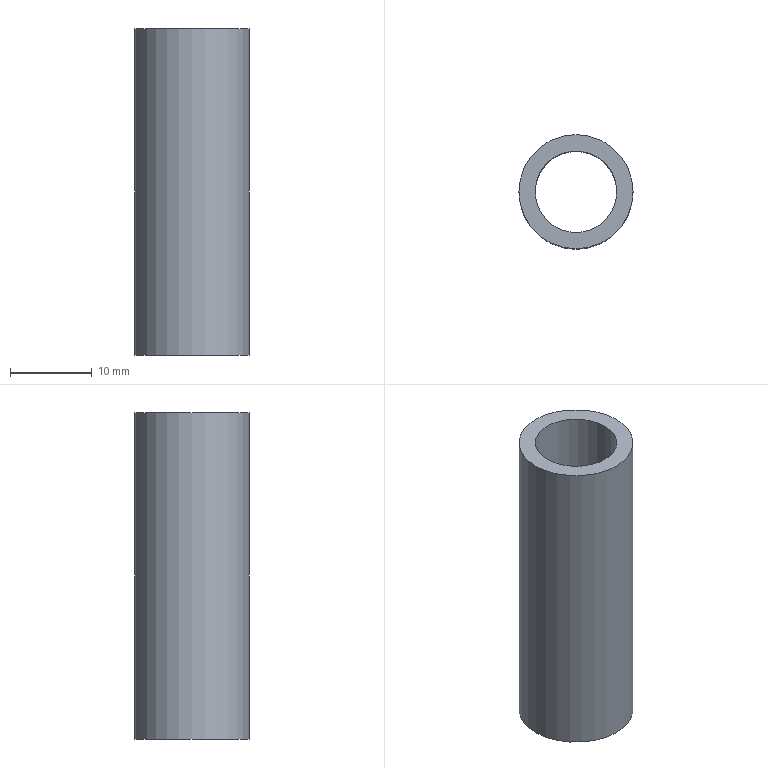Part | NX | features solid 2 | 1 solid | 4 faces | box 14 x 14 x 40 mm | volume 3016 mm3 | cylinder 2 | plane 2 | commonest cylinder face diameters 10 x1 14 x1
STEP:
#1=CARTESIAN_POINT('',(-1230.,410.,3.));
#2=VERTEX_POINT('',#1);
#3=CARTESIAN_POINT('',(-1225.,410.,3.));
#4=DIRECTION('',(0.,0.,-1.));
#5=DIRECTION('',(-1.,0.,0.));
#6=AXIS2_PLACEMENT_3D('',#3,#4,#5);
#7=CIRCLE('',#6,5.);
#8=EDGE_CURVE('',#2,#2,#7,.T.);
#9=ORIENTED_EDGE('',*,*,#8,.T.);
#10=EDGE_LOOP('',(#9));
#11=FACE_BOUND('',#10,.T.);
#12=CARTESIAN_POINT('',(-1230.,410.,43.));
#13=VERTEX_POINT('',#12);
#14=CARTESIAN_POINT('',(-1225.,410.,43.));
#15=DIRECTION('',(0.,0.,-1.));
#16=DIRECTION('',(-1.,0.,0.));
#17=AXIS2_PLACEMENT_3D('',#14,#15,#16);
#18=CIRCLE('',#17,5.);
#19=EDGE_CURVE('',#13,#13,#18,.T.);
#20=ORIENTED_EDGE('',*,*,#19,.F.);
#21=EDGE_LOOP('',(#20));
#22=FACE_BOUND('',#21,.T.);
#23=CARTESIAN_POINT('',(-1225.,410.,43.));
#24=DIRECTION('',(0.,0.,-1.));
#25=DIRECTION('',(-1.,0.,0.));
#26=AXIS2_PLACEMENT_3D('',#23,#24,#25);
#27=CYLINDRICAL_SURFACE('',#26,5.);
#28=ADVANCED_FACE('',(#11,#22),#27,.F.);
#29=ORIENTED_EDGE('',*,*,#19,.T.);
#30=EDGE_LOOP('',(#29));
#31=FACE_BOUND('',#30,.T.);
#32=CARTESIAN_POINT('',(-1232.,410.,43.));
#33=VERTEX_POINT('',#32);
#34=CARTESIAN_POINT('',(-1225.,410.,43.));
#35=DIRECTION('',(0.,0.,-1.));
#36=DIRECTION('',(-1.,0.,0.));
#37=AXIS2_PLACEMENT_3D('',#34,#35,#36);
#38=CIRCLE('',#37,7.);
#39=EDGE_CURVE('',#33,#33,#38,.T.);
#40=ORIENTED_EDGE('',*,*,#39,.F.);
#41=EDGE_LOOP('',(#40));
#42=FACE_BOUND('',#41,.T.);
#43=CARTESIAN_POINT('',(-1225.,410.,43.));
#44=DIRECTION('',(0.,0.,1.));
#45=DIRECTION('',(1.,0.,0.));
#46=AXIS2_PLACEMENT_3D('',#43,#44,#45);
#47=PLANE('',#46);
#48=ADVANCED_FACE('',(#31,#42),#47,.T.);
#49=ORIENTED_EDGE('',*,*,#8,.F.);
#50=EDGE_LOOP('',(#49));
#51=FACE_BOUND('',#50,.T.);
#52=CARTESIAN_POINT('',(-1232.,410.,3.));
#53=VERTEX_POINT('',#52);
#54=CARTESIAN_POINT('',(-1225.,410.,3.));
#55=DIRECTION('',(0.,0.,-1.));
#56=DIRECTION('',(-1.,0.,0.));
#57=AXIS2_PLACEMENT_3D('',#54,#55,#56);
#58=CIRCLE('',#57,7.);
#59=EDGE_CURVE('',#53,#53,#58,.T.);
#60=ORIENTED_EDGE('',*,*,#59,.T.);
#61=EDGE_LOOP('',(#60));
#62=FACE_BOUND('',#61,.T.);
#63=CARTESIAN_POINT('',(-1225.,410.,3.));
#64=DIRECTION('',(0.,0.,1.));
#65=DIRECTION('',(1.,0.,0.));
#66=AXIS2_PLACEMENT_3D('',#63,#64,#65);
#67=PLANE('',#66);
#68=ADVANCED_FACE('',(#51,#62),#67,.F.);
#69=ORIENTED_EDGE('',*,*,#59,.F.);
#70=EDGE_LOOP('',(#69));
#71=FACE_BOUND('',#70,.T.);
#72=ORIENTED_EDGE('',*,*,#39,.T.);
#73=EDGE_LOOP('',(#72));
#74=FACE_BOUND('',#73,.T.);
#75=CARTESIAN_POINT('',(-1225.,410.,43.));
#76=DIRECTION('',(0.,0.,-1.));
#77=DIRECTION('',(-1.,0.,0.));
#78=AXIS2_PLACEMENT_3D('',#75,#76,#77);
#79=CYLINDRICAL_SURFACE('',#78,7.);
#80=ADVANCED_FACE('',(#71,#74),#79,.T.);
#81=CLOSED_SHELL('',(#28,#48,#68,#80));
#82=MANIFOLD_SOLID_BREP('',#81);
#83=(LENGTH_UNIT()NAMED_UNIT(*)SI_UNIT(.MILLI.,.METRE.));
#84=UNCERTAINTY_MEASURE_WITH_UNIT(LENGTH_MEASURE(0.00001),#83,'','');
#85=(NAMED_UNIT(*)PLANE_ANGLE_UNIT()SI_UNIT($,.RADIAN.));
#86=(NAMED_UNIT(*)SI_UNIT($,.STERADIAN.)SOLID_ANGLE_UNIT());
#87=(GEOMETRIC_REPRESENTATION_CONTEXT(3)GLOBAL_UNCERTAINTY_ASSIGNED_CONTEXT((#84))GLOBAL_UNIT_ASSIGNED_CONTEXT((#83,#85,#86))REPRESENTATION_CONTEXT('',''));
#88=ADVANCED_BREP_SHAPE_REPRESENTATION('',(#82),#87);